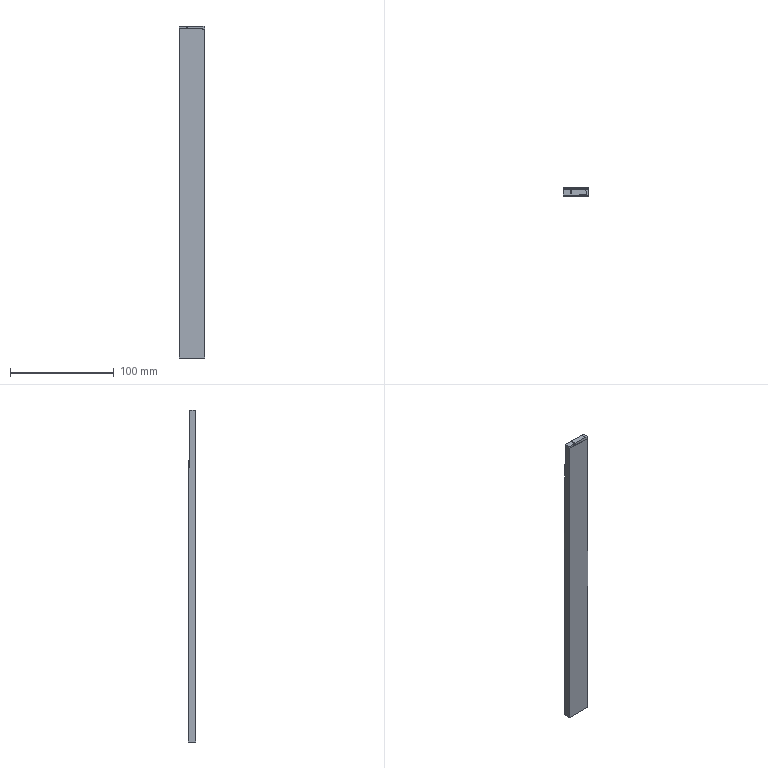Part | STEP file | P011002L005-000 | 1 solid | 91 faces | box 25 x 7.509 x 319.656 mm | volume 57786 mm3 | plane 51 | spline 12 | cone 10 | other 10 | cylinder 8 | commonest cylinder face diameters 4.048 x2 4.167 x2 4.983 x2 5 x2